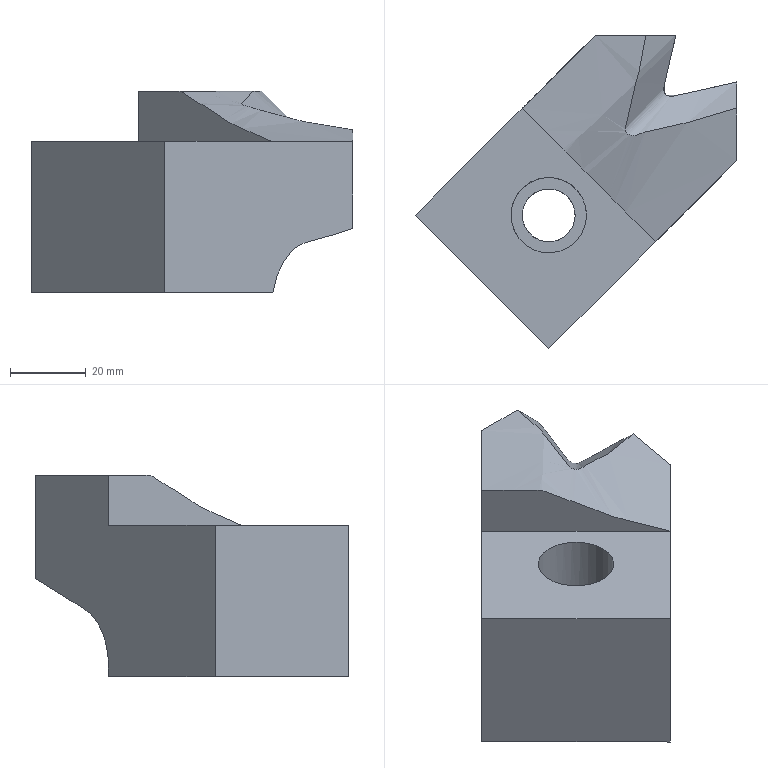Part | NX | features solid 2 | 1 solid | 28 faces | box 85.14 x 83.008 x 53.266 mm | volume 112514 mm3 | spline 18 | plane 8 | cylinder 2 | commonest cylinder face diameters 14 x1 20 x1